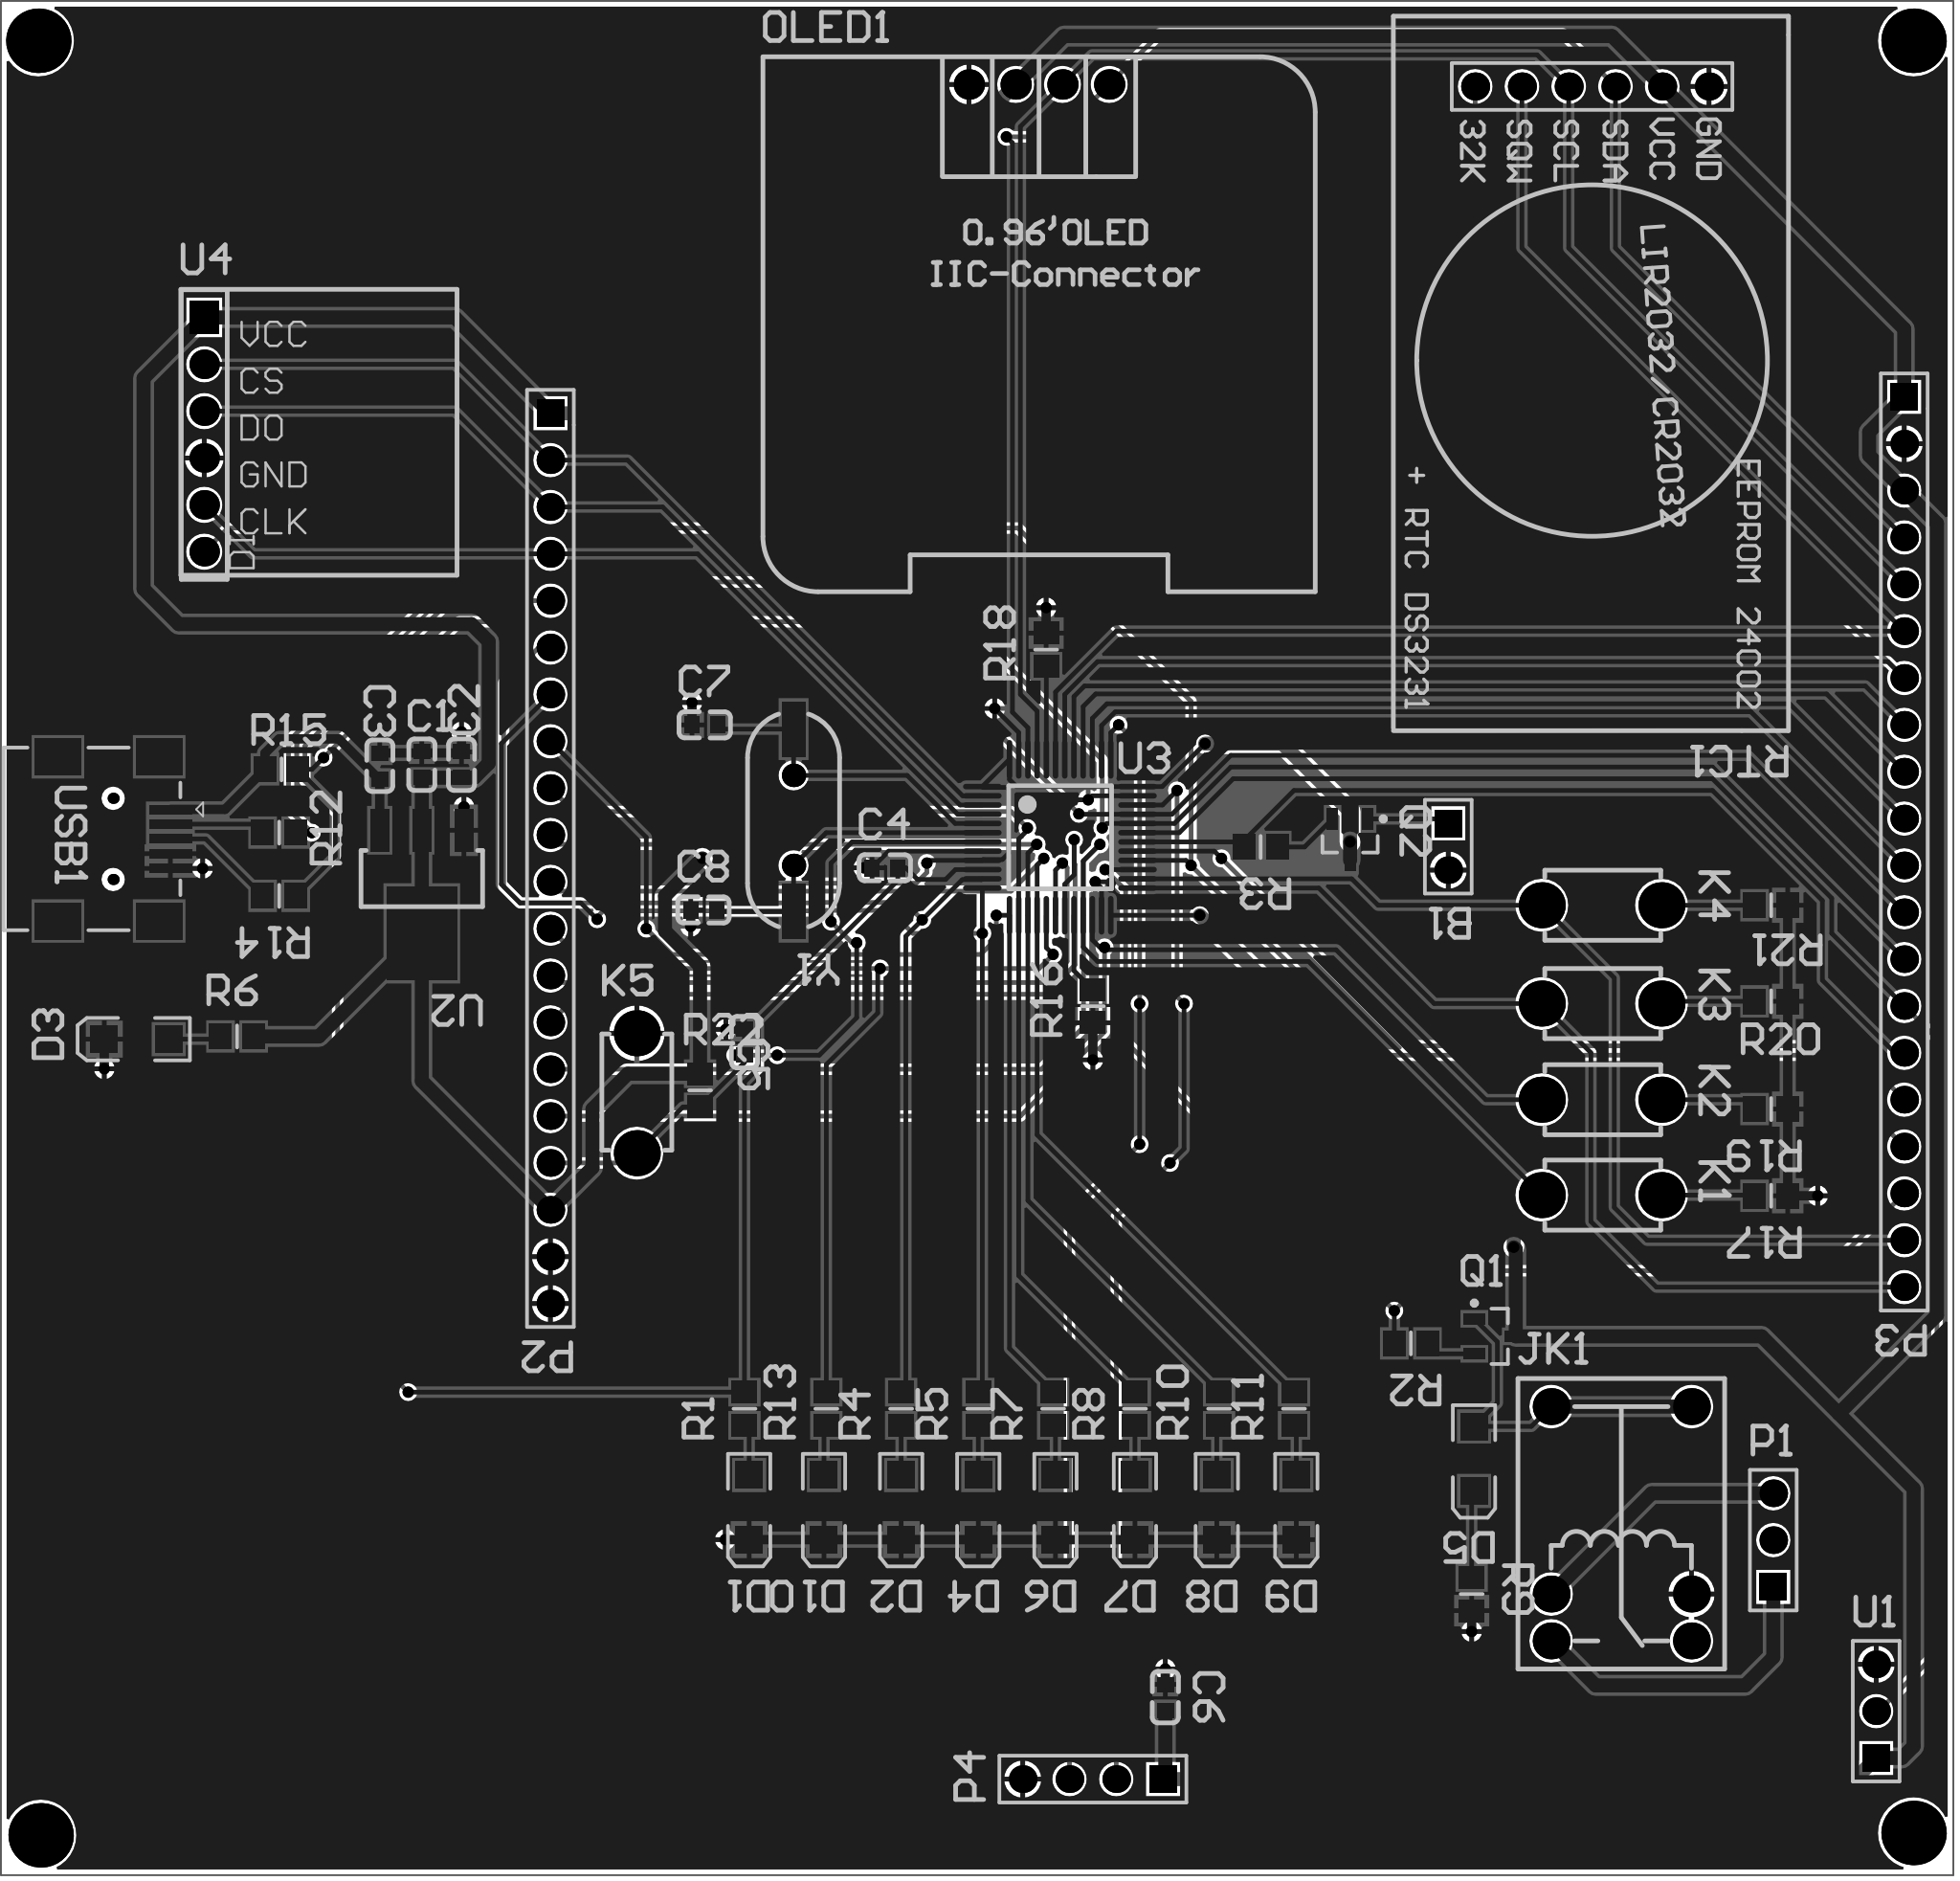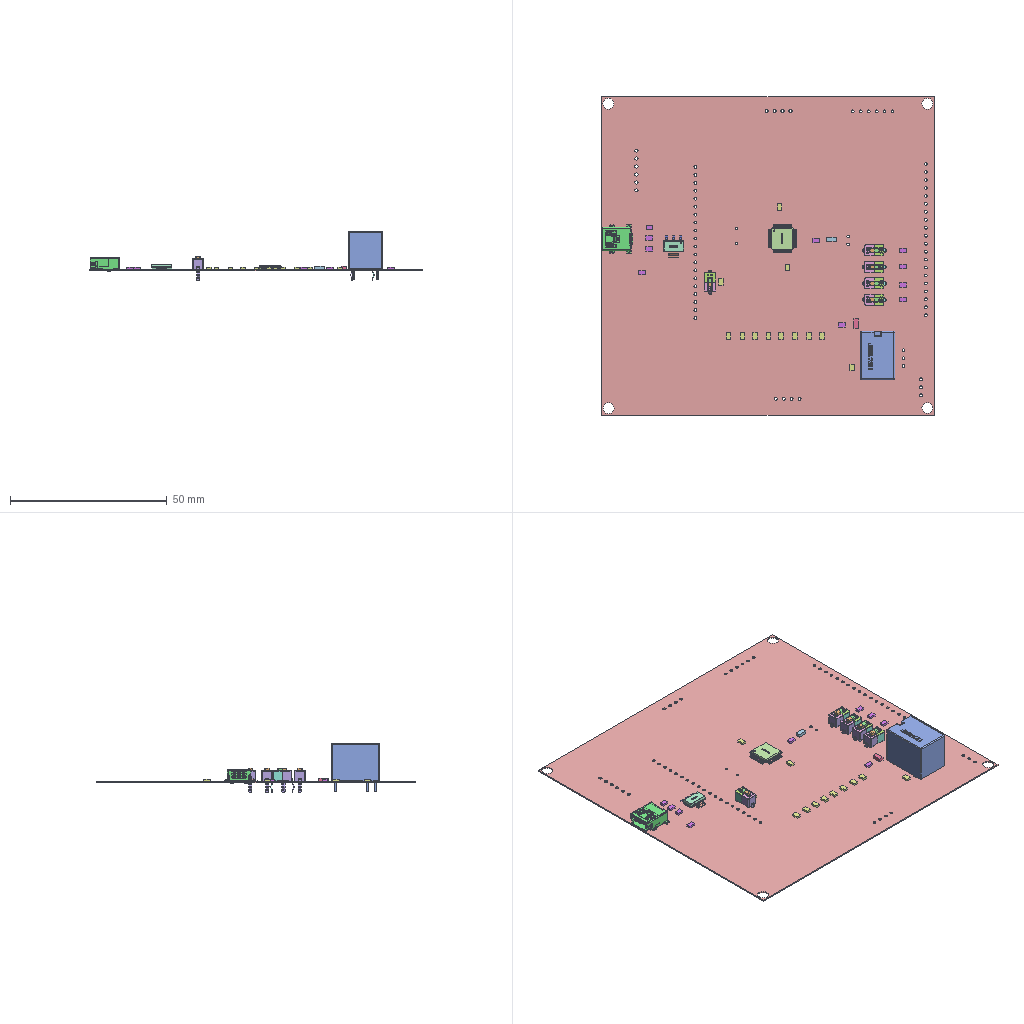Circuit board layout | Altium Designer | box 106 x 101.6 x 15.7 mm
Layer stack:
# Altium Designer layer stack of  (unit mm; dielectric type: 0 none, 1 core, 2 prepreg, 3 surface material)
index,name,kind,layer,copper_thickness_mm,dielectric_type,dielectric_thickness_mm,dielectric_material,dielectric_constant
0,Top Paste,other,,,,,,
1,Top Overlay,other,,,,,,
2,Top Solder,dielectric,,,3,0.0102,Solder Resist,3.5
3,Top Layer,copper,Top Layer,0.0356,,,,
4,Dielectric 1,dielectric,,,0,0.32,FR-4,4.8
5,Bottom Layer,copper,Bottom Layer,0.0356,,,,
6,Bottom Solder,dielectric,,,3,0.0102,Solder Resist,3.5
7,Bottom Overlay,other,,,,,,
8,Bottom Paste,other,,,,,,
# drill layer pairs: low layer,high layer
drill_pair,Top Layer,Bottom Layer
Part placement:
Designator,Comment,Layer,Footprint,Center-X(mm),Center-Y(mm),Rotation
B1,BEEP,TopLayer,HDR1X2,104.013,81.153,270
C1,10uF,TopLayer,C0603,48.257,85.59,270
C2,0.1uF,TopLayer,C0603,50.416,85.59,270
C3,10uF,TopLayer,C0603,45.974,85.533,270
C4,0.1uF,TopLayer,C0603,73.414,80.007,0
C5,0.1uF,TopLayer,C0603,65.786,70.55,270
C6,100NF,TopLayer,C0603,88.643,35.044,270
C7,20pF,TopLayer,C0603,63.635,87.754,0
C8,20pF,TopLayer,C0603,63.565,77.724,0
D1,POWER,TopLayer,3.2X1.6X1.1,66.04,45.339,270
D2,POWER,TopLayer,3.2X1.6X1.1,74.295,45.339,270
D3,POWER,TopLayer,3.2X1.6X1.1,32.764,70.719,180
D4,POWER,TopLayer,3.2X1.6X1.1,78.486,45.339,270
D5,POWER,TopLayer,3.2X1.6X1.1,105.41,47.978,270
D6,POWER,TopLayer,3.2X1.6X1.1,82.677,45.339,270
D7,POWER,TopLayer,3.2X1.6X1.1,86.995,45.339,270
D8,POWER,TopLayer,3.2X1.6X1.1,91.44,45.339,270
D9,POWER,TopLayer,3.2X1.6X1.1,95.758,45.339,270
D10,POWER,TopLayer,3.2X1.6X1.1,70.104,45.339,270
JK1,HK4100F-DC5V-SHG,TopLayer,HK4100F,113.411,44.45,90
K1,KEY,TopLayer,DIP-3X6X4.3,112.343,62.265,360
K2,KEY,TopLayer,DIP-3X6X4.3,112.343,67.437,360
K3,KEY,TopLayer,DIP-3X6X4.3,112.343,72.649,360
K4,KEY,TopLayer,DIP-3X6X4.3,112.343,77.978,360
K5,KEY,TopLayer,DIP-3X6X4.3,59.939,67.788,90
OLED1,0.96OLED_4P_MODULE_JX,TopLayer,0.96OLED_4P,81.787,122.473,0
P1,Header 3,TopLayer,HDR1X3,121.666,43.561,90
P2,Header 20,TopLayer,HDR1X20,55.245,80.518,270
P3,Header 20,TopLayer,HDR1X20,128.778,81.407,270
P4,Header 4,TopLayer,HDR1X4,84.709,30.607,180
Q1,PNP,TopLayer,SOT-23B_N,106.553,54.61,360
Q2,PNP,TopLayer,SOT-23B_N,98.679,81.534,270
R1,330,TopLayer,6-0805_N,65.786,50.684,90
R2,1K,TopLayer,6-0805_N,101.981,54.229,180
R3,4.7K,TopLayer,6-0805_N,93.822,81.137,180
R4,330,TopLayer,6-0805_N,74.295,50.684,90
R5,330,TopLayer,6-0805_N,78.486,50.684,90
R6,330,TopLayer,6-0805_N,38.227,70.866,360
R7,330,TopLayer,6-0805_N,82.55,50.684,90
R8,330,TopLayer,6-0805_N,86.995,50.684,90
R9,1K,TopLayer,6-0805_N,105.283,40.64,270
R10,330,TopLayer,6-0805_N,91.567,50.684,90
R11,330,TopLayer,6-0805_N,95.631,50.684,90
R12,100,TopLayer,6-0805_N,40.513,81.915,180
R13,330,TopLayer,6-0805_N,70.231,50.684,90
R14,100,TopLayer,6-0805_N,40.513,78.486,180
R15,10K,TopLayer,6-0805_N,40.64,85.344,180
R16,10K,TopLayer,6-0805_N,84.709,72.506,90
R17,10K,TopLayer,6-0805_N,121.55,62.23,180
R18,10K,TopLayer,6-0805_N,82.169,91.832,90
R19,10K,TopLayer,6-0805_N,121.55,66.929,180
R20,10K,TopLayer,6-0805_N,121.55,72.771,180
R21,10K,TopLayer,6-0805_N,121.55,77.978,180
R22,10K,TopLayer,6-0805_N,63.373,67.945,90
RTC1,DS3231-RTC-SINGLE-HEADER,TopLayer,DS3231-RTC-24C32-EEPROM-SINGLE-HEADER,111.823,122.365,270
U1,DHT11,TopLayer,HDR1X3,127.254,34.29,90
U2,AMS1117,TopLayer,SOT223,48.26,79.248,180
U3,STM32F103C8T6,TopLayer,LQFP48_7X7,82.918,81.661,270
U4,W25Q128  SPI-Flash外部存储器,TopLayer,SPI_FLASH,36.442,103.493,360
USB1,MINI-USB,TopLayer,USB-MINI-A,31.55,81.575,270
Y1,12M,TopLayer,XTAL_US,68.453,82.577,270
Pad and via stacks:
# Altium Designer via and pad stacks of  (unit mm). Each distinct definition once, with the count of objects using it.
# via: kind,start_layer,end_layer,hole_mm,diameter_mm,mode(0 simple;1 top-mid-bottom;2 full stack),diameter_per_layer,count,example_net
# pad: kind,layer,hole_mm,hole_type(0 round;1 square;2 slot),plating,top_size,top_shape(1 round;2 rect;3 octagon;9 rounded rect),mid_size,bottom_size,mode,footprint,size_per_layer,count,example
pad,Multi-Layer,3.5,0,plated,3.5x3.5,1,3.5x3.5,3.5x3.5,0,,,4,5
pad,Multi-Layer,0.9,0,plated,1.5x1.5,2,1.5x1.5,1.5x1.5,0,HDR1X4,,1,P4.1
pad,Multi-Layer,0.9,0,plated,1.5x1.5,1,1.5x1.5,1.5x1.5,0,HDR1X4,,3,P4.2
pad,Multi-Layer,0.7112,0,plated,1.27x1.27,1,1.27x1.27,1.27x1.27,0,XTAL_US,,2,Y1.1
pad,Multi-Layer,1.2,0,plated,2.5x2.5,1,2.5x2.5,2.5x2.5,0,DIP-3X6X4.3,,10,K5.3
pad,Multi-Layer,0.9,0,plated,1.5x1.5,1,1.5x1.5,1.5x1.5,0,HDR1X20,,38,P2.20
pad,Multi-Layer,0.9,0,plated,1.5x1.5,2,1.5x1.5,1.5x1.5,0,HDR1X20,,2,P2.1
pad,Multi-Layer,1,2,plated,1.65x1.65,1,1.65x1.65,1.65x1.65,0,0.96OLED_4P,,4,OLED1.4
pad,Multi-Layer,1.02,0,plated,1.6x1.6,1,1.6x1.6,1.6x1.6,0,SPI FLASH,,5,U4.6
pad,Multi-Layer,1.02,0,plated,1.8x1.6,2,1.8x1.6,1.8x1.6,0,SPI FLASH,,1,U4.1
pad,Multi-Layer,0.9144,2,plated,1.524x1.524,1,1.524x1.524,1.524x1.524,0,DS3231-RTC-24C32-EEPROM-SINGLE-HEADER,,6,RTC1.6
pad,Multi-Layer,0.9,0,unplated,0.6x0.6,1,0.6x0.6,0.6x0.6,0,USB-MINI-A,,2,USB1.MH2
pad,Multi-Layer,0.9,0,plated,1.5x1.5,1,1.5x1.5,1.5x1.5,0,HDR1X2,,1,B1.2
pad,Multi-Layer,0.9,0,plated,1.5x1.5,2,1.5x1.5,1.5x1.5,0,HDR1X2,,1,B1.1
pad,Multi-Layer,0.9,0,plated,1.5x1.5,1,1.5x1.5,1.5x1.5,0,HDR1X3,,4,P1.3
pad,Multi-Layer,0.9,0,plated,1.5x1.5,2,1.5x1.5,1.5x1.5,0,HDR1X3,,2,P1.1
pad,Multi-Layer,1,0,plated,2x2,1,2x2,2x2,0,HK4100F,,6,JK1.2
pad,Top Layer,0,0,plated,0.8x0.9,2,0.8x0.9,0.8x0.9,0,C0603,,16,C7.2
pad,Top Layer,0,0,plated,1.4x1.2,2,1.4x1.2,1.4x1.2,0,6-0805_N,,44,R22.2
pad,Top Layer,0,0,plated,3x1.27,2,3x1.27,3x1.27,0,XTAL_US,,2,Y1.1
pad,Top Layer,0,0,plated,0.3x2.1,1,0.3x2.1,0.3x2.1,0,LQFP48 7X7,,48,U3.1
pad,Top Layer,0,0,plated,3.81x5.08,2,3.81x5.08,3.81x5.08,0,SOT223,,1,U2.2
pad,Top Layer,0,0,plated,1.016x2.286,2,1.016x2.286,1.016x2.286,0,SOT223,,3,U2.2
pad,Top Layer,0,0,plated,1.5x1.5,2,1.5x1.5,1.5x1.5,0,3.2X1.6X1.1,,20,D10.2
pad,Top Layer,0,0,plated,2x2.5,2,2x2.5,2x2.5,0,USB-MINI-A,,4,USB1.0
pad,Top Layer,0,0,plated,0.5x2.3,2,0.5x2.3,0.5x2.3,0,USB-MINI-A,,5,USB1.5
pad,Top Layer,0,0,plated,0.6x1.15,2,0.6x1.15,0.6x1.15,0,SOT-23B_N,,6,Q2.3
via,Top Layer,Bottom Layer,0.3048,0.6096,0,,57,3V3
Copper pours:
name,layer,net,type(0 solid;1 hatched;2 none)
G,Top Layer,GND,0
G,Bottom Layer,GND,0
Design rules, without the lines most boards share:
# Altium Designer design rules of  (exported by Altium Designer, unit mm)
# columns: name | kind | enabled | priority | scope1 | scope2 | descriptor | typed fields (field=value)
NetAntennae | 56 | enabled | 1 | All | All | Net Antennae (Tolerance=0mm) (All) |
SilkToSilkClearance | 55 | enabled | 1 | All | All | Silk to Silk (Clearance=0mm) (All),(All) |
SilkToSolderMaskClearance | 54 | enabled | 1 | IsPad | All | Silk To Solder Mask (Clearance=0mm) (IsPad),(All) |
MinimumSolderMaskSliver | 53 | enabled | 1 | All | All | Minimum Solder Mask Sliver (Gap=0mm) (All),(All) |
HoleToHoleClearance | 52 | enabled | 1 | All | All | Hole To Hole Clearance (Gap=0.254mm) (All),(All) | gap=0.254
DiffPairsRouting | 51 | enabled | 1 | All | All | Differential Pairs Uncoupled Length using the Gap Constraints (Min=0.254mm) (Max=0.254mm) (Prefered=0.254mm)  and Width Constraints (Min=0.381mm) (Max=0.381mm) (Prefered=0.381mm) (All) |
HoleSize | 42 | enabled | 1 | All | All | Hole Size Constraint (Min=0.025mm) (Max=2.54mm) (All) |
Height | 50 | enabled | 1 | All | All | Height Constraint (Min=0mm) (Max=25.4mm) (Prefered=12.7mm) (All) | min_height=0 max_height=25.4
ComponentClearance | 24 | enabled | 1 | All | All | Component Clearance Constraint ( Horizontal Gap = 0.254mm, Vertical Gap = 0.254mm ) (All),(All)  | gap=0.254
SolderMaskExpansion | 13 | enabled | 1 | All | All | Solder Mask Expansion (Expansion =0.102mm) (All) | expansion=0.1016
PasteMaskExpansion | 14 | enabled | 1 | All | All | Paste Mask Expansion (Expansion =0mm) (All) | expansion=0
RoutingVias | 11 | enabled | 1 | All | All | Routing Via (MinHoleWidth=0.711mm) (MaxHoleWidth=0.711mm) (PreferredHoleWidth=0.711mm) (MinWidth=1.27mm) (MaxWidth=1.27mm) (PreferedWidth=1.27mm) (All) | via_min_hole=0.7112 via_max_hole=0.7112 via_preferred_diameter=1.27 via_preferred_hole=0.7112
RoutingCorners | 10 | enabled | 1 | All | All | Routing Corners (Style=45-Degree) (Min Setback=2.54mm) (Max Setback=2.54mm) (All) |
Width | 2 | enabled | 1 | All | All | Width Constraint (Min=0.254mm) (Max=0.762mm) (Preferred=0.254mm) (All) |
PolygonConnect | 20 | enabled | 1 | All | All | Polygon Connect Rule(Relief Connect )(Conductor Width=0.254mm) (Relief Angle=90 Angle) (Entries=4) (Air Gap Width=0.254mm) (All),(All) | connect_style(0=relief,1=direct,2=none)=0 relief_conductor_width=0.254 relief_entries=4
PlaneClearance | 12 | enabled | 1 | All | All | Power Plane Clearance (Clearance =0.508mm) (All) | clearance=0.508
PlaneConnect | 6 | enabled | 1 | All | All | Power Plane Connect Rule(Relief Connect )(Expansion=0.508mm) (Conductor Width=0.254mm) (Air Gap=0.254mm) (Entries=4) (All) | relief_conductor_width=0.254 relief_entries=4 relief_expansion=0.508
Clearance | 0 | enabled | 1 | All | All | Clearance Constraint (Gap=0.178mm) (All),(All) | gap=0.1778
Classes set for this board:
# Altium Designer classes of  (member kind: 0 net, 1 component, 2 from-to, 3 pad, 4 layer, 5 differential pair, 6 design channel, 7 polygon, 8 structure, 9 xSignal)
# columns: class name | member kind | superclass | members
Sheet2 | 1 | no | B1; C1; C2; C3; C4; C5; C6; C7; C8; D1; D2; D3; D4; D5; D6; D7; D8; D9; D10; JK1; K1; K2; K3; K4; K5; OLED1; P1; P2; P3; P4; Q1; Q2; R1; R2; R3; R4; R5; R6; R7; R8; R9; R10; R11; R12; R13; R14; R15; R16; R17; R18; R19; R20; R21; R22; RTC1; U1; U2; U3; U4; USB1; Y1;